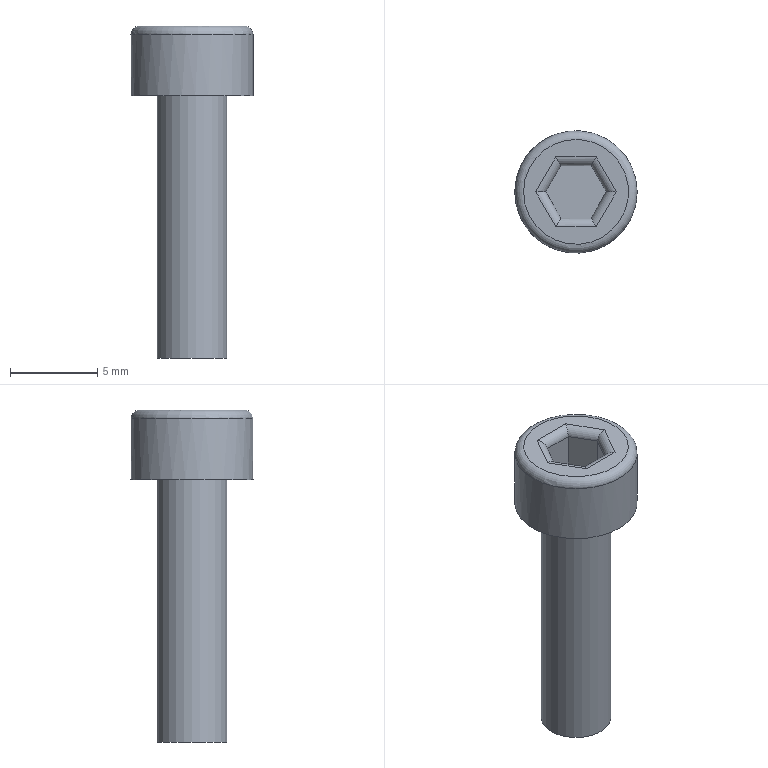Part | STEP file | Tube feed_id634_x_t | 1 solid | 19 faces | box 7 x 7 x 19 mm | volume 320.116 mm3 | plane 10 | cylinder 8 | torus 1 | commonest cylinder face diameters 1 x6 4 x1 7 x1